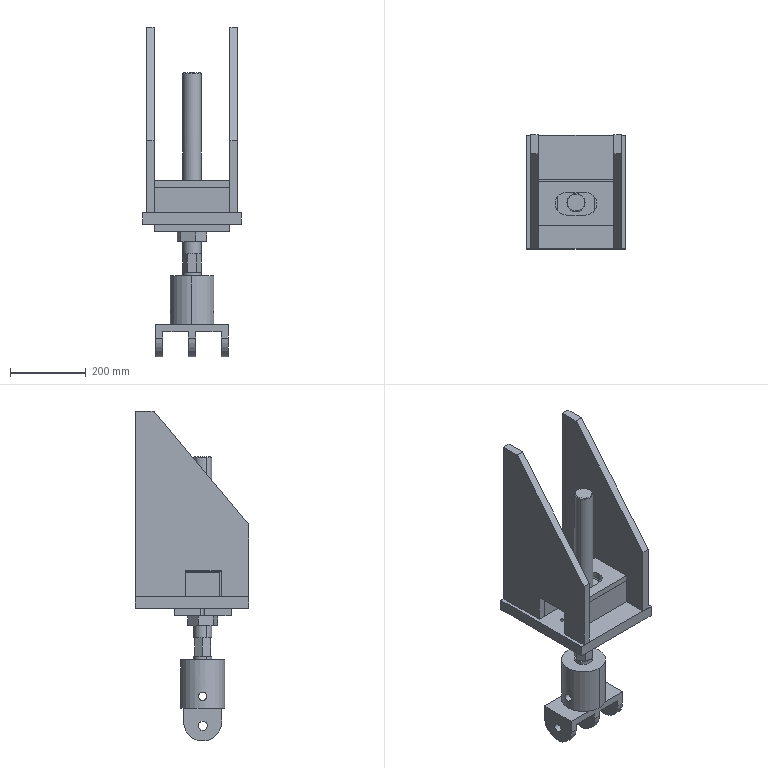Part | SolidWorks | 13 solids | 177 faces | box 260 x 300 x 870.542 mm | volume 11020078 mm3 | plane 116 | cylinder 55 | cone 6 | commonest cylinder face diameters 48 x12 22 x6 24 x6 60 x6 76 x6 10.2 x4